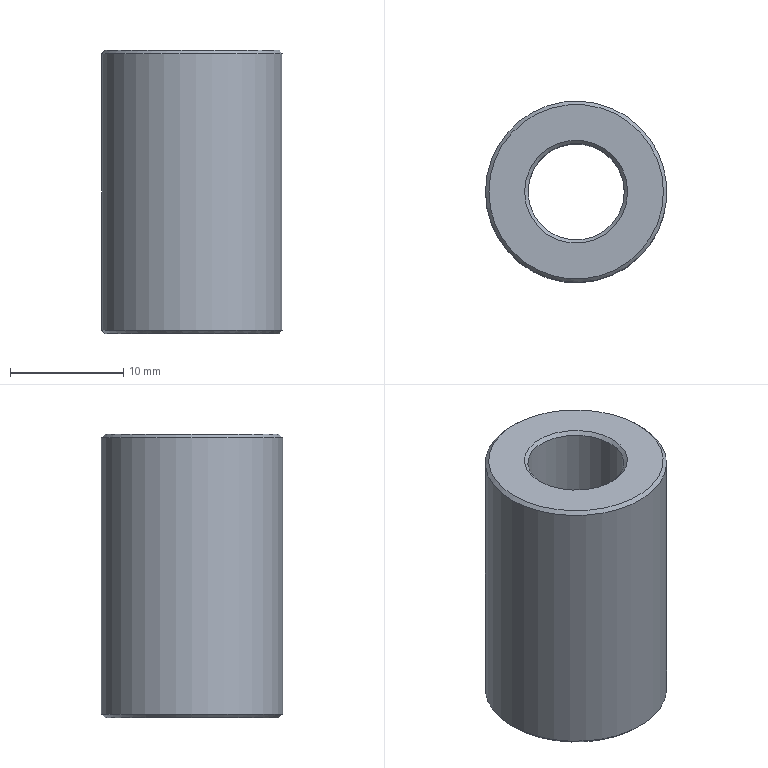Part | STEP file | 200 mesh_id166_x | 1 solid | 8 faces | box 16 x 16 x 25 mm | volume 3601 mm3 | cone 4 | cylinder 2 | plane 2 | commonest cylinder face diameters 8.5 x1 16 x1
STEP:
#1=CARTESIAN_POINT('',(-17065.884,-3985.269,87.558));
#2=VERTEX_POINT('',#1);
#3=CARTESIAN_POINT('',(-17057.884,-3985.269,87.558));
#4=DIRECTION('',(0.,0.,1.));
#5=DIRECTION('',(-1.,0.,0.));
#6=AXIS2_PLACEMENT_3D('',#3,#4,#5);
#7=CIRCLE('',#6,8.);
#8=EDGE_CURVE('',#2,#2,#7,.T.);
#9=ORIENTED_EDGE('',*,*,#8,.T.);
#10=EDGE_LOOP('',(#9));
#11=FACE_BOUND('',#10,.T.);
#12=CARTESIAN_POINT('',(-17065.884,-3985.269,111.958));
#13=VERTEX_POINT('',#12);
#14=CARTESIAN_POINT('',(-17057.884,-3985.269,111.958));
#15=DIRECTION('',(0.,0.,-1.));
#16=DIRECTION('',(-1.,0.,0.));
#17=AXIS2_PLACEMENT_3D('',#14,#15,#16);
#18=CIRCLE('',#17,8.);
#19=EDGE_CURVE('',#13,#13,#18,.T.);
#20=ORIENTED_EDGE('',*,*,#19,.T.);
#21=EDGE_LOOP('',(#20));
#22=FACE_BOUND('',#21,.T.);
#23=CARTESIAN_POINT('',(-17057.884,-3985.269,85.258));
#24=DIRECTION('',(0.,0.,1.));
#25=DIRECTION('',(1.,0.,0.));
#26=AXIS2_PLACEMENT_3D('',#23,#24,#25);
#27=CYLINDRICAL_SURFACE('',#26,8.);
#28=ADVANCED_FACE('',(#11,#22),#27,.T.);
#29=CARTESIAN_POINT('',(-17065.584,-3985.269,87.258));
#30=VERTEX_POINT('',#29);
#31=CARTESIAN_POINT('',(-17057.884,-3985.269,87.258));
#32=DIRECTION('',(0.,0.,-1.));
#33=DIRECTION('',(-1.,0.,0.));
#34=AXIS2_PLACEMENT_3D('',#31,#32,#33);
#35=CIRCLE('',#34,7.7);
#36=EDGE_CURVE('',#30,#30,#35,.T.);
#37=ORIENTED_EDGE('',*,*,#36,.T.);
#38=EDGE_LOOP('',(#37));
#39=FACE_BOUND('',#38,.T.);
#40=CARTESIAN_POINT('',(-17062.434,-3985.269,87.258));
#41=VERTEX_POINT('',#40);
#42=CARTESIAN_POINT('',(-17057.884,-3985.269,87.258));
#43=DIRECTION('',(0.,0.,1.));
#44=DIRECTION('',(-1.,0.,0.));
#45=AXIS2_PLACEMENT_3D('',#42,#43,#44);
#46=CIRCLE('',#45,4.55);
#47=EDGE_CURVE('',#41,#41,#46,.T.);
#48=ORIENTED_EDGE('',*,*,#47,.T.);
#49=EDGE_LOOP('',(#48));
#50=FACE_BOUND('',#49,.T.);
#51=CARTESIAN_POINT('',(-17057.884,-3985.269,87.258));
#52=DIRECTION('',(0.,0.,-1.));
#53=DIRECTION('',(1.,0.,0.));
#54=AXIS2_PLACEMENT_3D('',#51,#52,#53);
#55=PLANE('',#54);
#56=ADVANCED_FACE('',(#39,#50),#55,.T.);
#57=CARTESIAN_POINT('',(-17062.134,-3985.269,87.558));
#58=VERTEX_POINT('',#57);
#59=CARTESIAN_POINT('',(-17057.884,-3985.269,87.558));
#60=DIRECTION('',(0.,0.,-1.));
#61=DIRECTION('',(-1.,0.,0.));
#62=AXIS2_PLACEMENT_3D('',#59,#60,#61);
#63=CIRCLE('',#62,4.25);
#64=EDGE_CURVE('',#58,#58,#63,.T.);
#65=ORIENTED_EDGE('',*,*,#64,.T.);
#66=EDGE_LOOP('',(#65));
#67=FACE_BOUND('',#66,.T.);
#68=CARTESIAN_POINT('',(-17062.134,-3985.269,111.958));
#69=VERTEX_POINT('',#68);
#70=CARTESIAN_POINT('',(-17057.884,-3985.269,111.958));
#71=DIRECTION('',(0.,0.,1.));
#72=DIRECTION('',(-1.,0.,0.));
#73=AXIS2_PLACEMENT_3D('',#70,#71,#72);
#74=CIRCLE('',#73,4.25);
#75=EDGE_CURVE('',#69,#69,#74,.T.);
#76=ORIENTED_EDGE('',*,*,#75,.T.);
#77=EDGE_LOOP('',(#76));
#78=FACE_BOUND('',#77,.T.);
#79=CARTESIAN_POINT('',(-17057.884,-3985.269,121.258));
#80=DIRECTION('',(0.,0.,-1.));
#81=DIRECTION('',(1.,0.,0.));
#82=AXIS2_PLACEMENT_3D('',#79,#80,#81);
#83=CYLINDRICAL_SURFACE('',#82,4.25);
#84=ADVANCED_FACE('',(#67,#78),#83,.F.);
#85=CARTESIAN_POINT('',(-17065.584,-3985.269,112.258));
#86=VERTEX_POINT('',#85);
#87=CARTESIAN_POINT('',(-17057.884,-3985.269,112.258));
#88=DIRECTION('',(0.,0.,1.));
#89=DIRECTION('',(-1.,0.,0.));
#90=AXIS2_PLACEMENT_3D('',#87,#88,#89);
#91=CIRCLE('',#90,7.7);
#92=EDGE_CURVE('',#86,#86,#91,.T.);
#93=ORIENTED_EDGE('',*,*,#92,.T.);
#94=EDGE_LOOP('',(#93));
#95=FACE_BOUND('',#94,.T.);
#96=CARTESIAN_POINT('',(-17062.434,-3985.269,112.258));
#97=VERTEX_POINT('',#96);
#98=CARTESIAN_POINT('',(-17057.884,-3985.269,112.258));
#99=DIRECTION('',(0.,0.,-1.));
#100=DIRECTION('',(-1.,0.,0.));
#101=AXIS2_PLACEMENT_3D('',#98,#99,#100);
#102=CIRCLE('',#101,4.55);
#103=EDGE_CURVE('',#97,#97,#102,.T.);
#104=ORIENTED_EDGE('',*,*,#103,.T.);
#105=EDGE_LOOP('',(#104));
#106=FACE_BOUND('',#105,.T.);
#107=CARTESIAN_POINT('',(-17057.884,-3985.269,112.258));
#108=DIRECTION('',(0.,0.,-1.));
#109=DIRECTION('',(-1.,0.,0.));
#110=AXIS2_PLACEMENT_3D('',#107,#108,#109);
#111=PLANE('',#110);
#112=ADVANCED_FACE('',(#95,#106),#111,.F.);
#113=ORIENTED_EDGE('',*,*,#19,.F.);
#114=EDGE_LOOP('',(#113));
#115=FACE_BOUND('',#114,.T.);
#116=ORIENTED_EDGE('',*,*,#92,.F.);
#117=EDGE_LOOP('',(#116));
#118=FACE_BOUND('',#117,.T.);
#119=CARTESIAN_POINT('',(-17057.884,-3985.269,112.258));
#120=DIRECTION('',(0.,0.,-1.));
#121=DIRECTION('',(-1.,0.,0.));
#122=AXIS2_PLACEMENT_3D('',#119,#120,#121);
#123=CONICAL_SURFACE('',#122,7.7,45.);
#124=ADVANCED_FACE('',(#115,#118),#123,.T.);
#125=ORIENTED_EDGE('',*,*,#103,.F.);
#126=EDGE_LOOP('',(#125));
#127=FACE_BOUND('',#126,.T.);
#128=ORIENTED_EDGE('',*,*,#75,.F.);
#129=EDGE_LOOP('',(#128));
#130=FACE_BOUND('',#129,.T.);
#131=CARTESIAN_POINT('',(-17057.884,-3985.269,111.958));
#132=DIRECTION('',(0.,0.,1.));
#133=DIRECTION('',(1.,0.,0.));
#134=AXIS2_PLACEMENT_3D('',#131,#132,#133);
#135=CONICAL_SURFACE('',#134,4.25,45.);
#136=ADVANCED_FACE('',(#127,#130),#135,.F.);
#137=ORIENTED_EDGE('',*,*,#47,.F.);
#138=EDGE_LOOP('',(#137));
#139=FACE_BOUND('',#138,.T.);
#140=ORIENTED_EDGE('',*,*,#64,.F.);
#141=EDGE_LOOP('',(#140));
#142=FACE_BOUND('',#141,.T.);
#143=CARTESIAN_POINT('',(-17057.884,-3985.269,87.558));
#144=DIRECTION('',(0.,0.,-1.));
#145=DIRECTION('',(-1.,0.,0.));
#146=AXIS2_PLACEMENT_3D('',#143,#144,#145);
#147=CONICAL_SURFACE('',#146,4.25,45.);
#148=ADVANCED_FACE('',(#139,#142),#147,.F.);
#149=ORIENTED_EDGE('',*,*,#36,.F.);
#150=EDGE_LOOP('',(#149));
#151=FACE_BOUND('',#150,.T.);
#152=ORIENTED_EDGE('',*,*,#8,.F.);
#153=EDGE_LOOP('',(#152));
#154=FACE_BOUND('',#153,.T.);
#155=CARTESIAN_POINT('',(-17057.884,-3985.269,87.558));
#156=DIRECTION('',(0.,0.,1.));
#157=DIRECTION('',(1.,0.,0.));
#158=AXIS2_PLACEMENT_3D('',#155,#156,#157);
#159=CONICAL_SURFACE('',#158,8.,45.);
#160=ADVANCED_FACE('',(#151,#154),#159,.T.);
#161=CLOSED_SHELL('',(#28,#56,#84,#112,#124,#136,#148,#160));
#162=MANIFOLD_SOLID_BREP('',#161);
#163=(LENGTH_UNIT()NAMED_UNIT(*)SI_UNIT(.MILLI.,.METRE.));
#164=UNCERTAINTY_MEASURE_WITH_UNIT(LENGTH_MEASURE(0.00002),#163,'','');
#165=(NAMED_UNIT(*)PLANE_ANGLE_UNIT()SI_UNIT($,.RADIAN.));
#166=PLANE_ANGLE_MEASURE_WITH_UNIT(PLANE_ANGLE_MEASURE(0.01745),#165);
#167=DIMENSIONAL_EXPONENTS(0.,0.,0.,0.,0.,0.,0.);
#168=(CONVERSION_BASED_UNIT('DEGREE',#166)NAMED_UNIT(#167)PLANE_ANGLE_UNIT());
#169=(NAMED_UNIT(*)SI_UNIT($,.STERADIAN.)SOLID_ANGLE_UNIT());
#170=(GEOMETRIC_REPRESENTATION_CONTEXT(3)GLOBAL_UNCERTAINTY_ASSIGNED_CONTEXT((#164))GLOBAL_UNIT_ASSIGNED_CONTEXT((#163,#168,#169))REPRESENTATION_CONTEXT('',''));
#171=ADVANCED_BREP_SHAPE_REPRESENTATION('',(#162),#170);